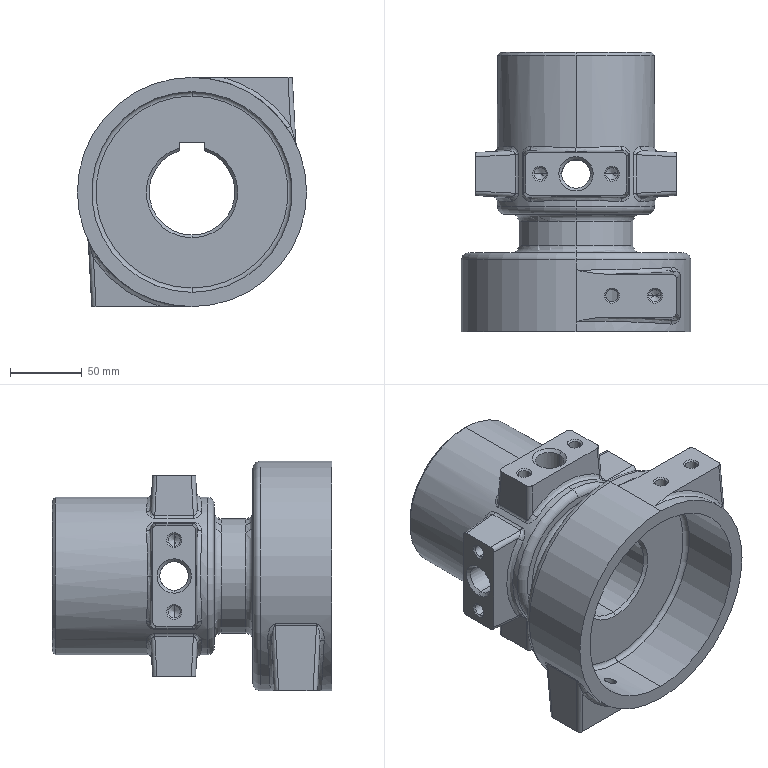Part | SolidWorks | features ICE 9, Chamfer 8, CirPattern 5, Fillet 3, HoleWzd 2, Revolution 1 | 1 solid | 224 faces | box 160 x 195 x 160 mm | volume 950128 mm3 | cylinder 76 | cone 60 | plane 42 | spline 36 | torus 10 | commonest cylinder face diameters 6 x30 8.5 x24 20 x8 60 x2 80 x2 90 x2